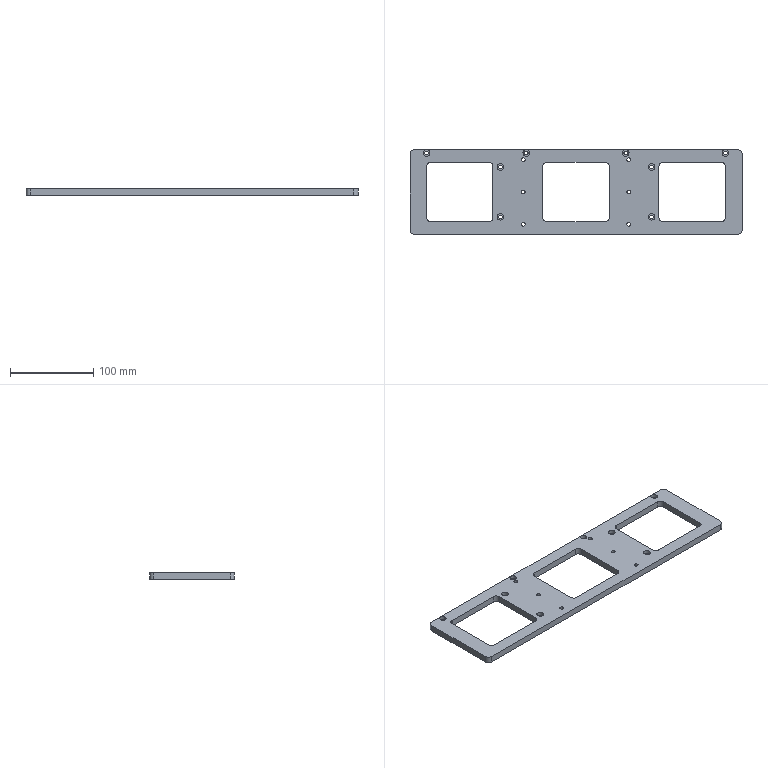Part | NX | 1 solid | 76 faces | box 400 x 102 x 8 mm | volume 184715 mm3 | cylinder 44 | plane 32 | commonest cylinder face diameters 10 x16 4.5 x14 7.8 x10 8 x4